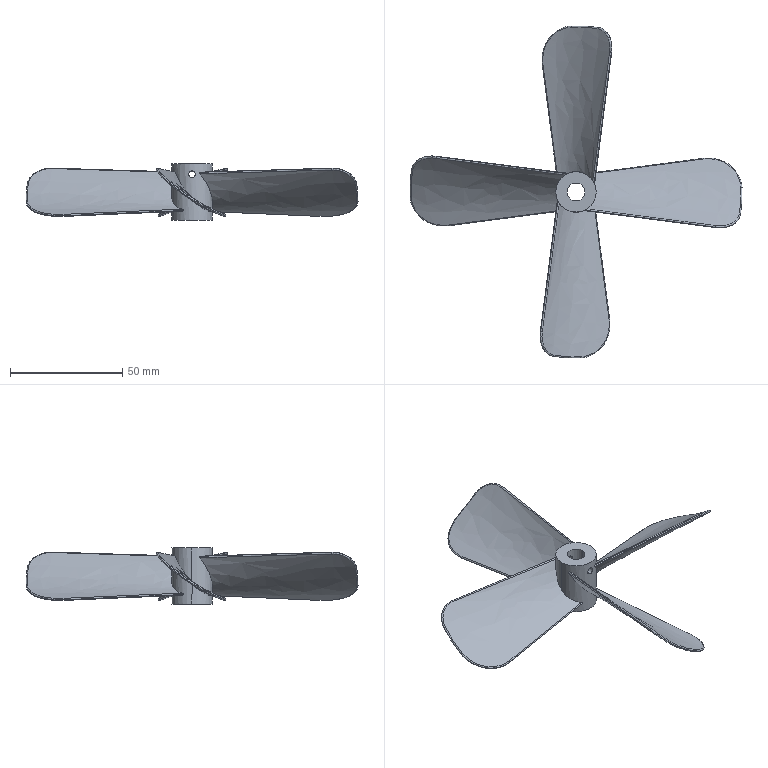Part | SolidWorks | features BaseBody 1 | 1 solid | 61 faces | box 147.93 x 147.93 x 25 mm | volume 13194 mm3 | spline 48 | cylinder 10 | plane 3 | commonest cylinder face diameters 3 x4 8 x2 9.26 x2 18 x2